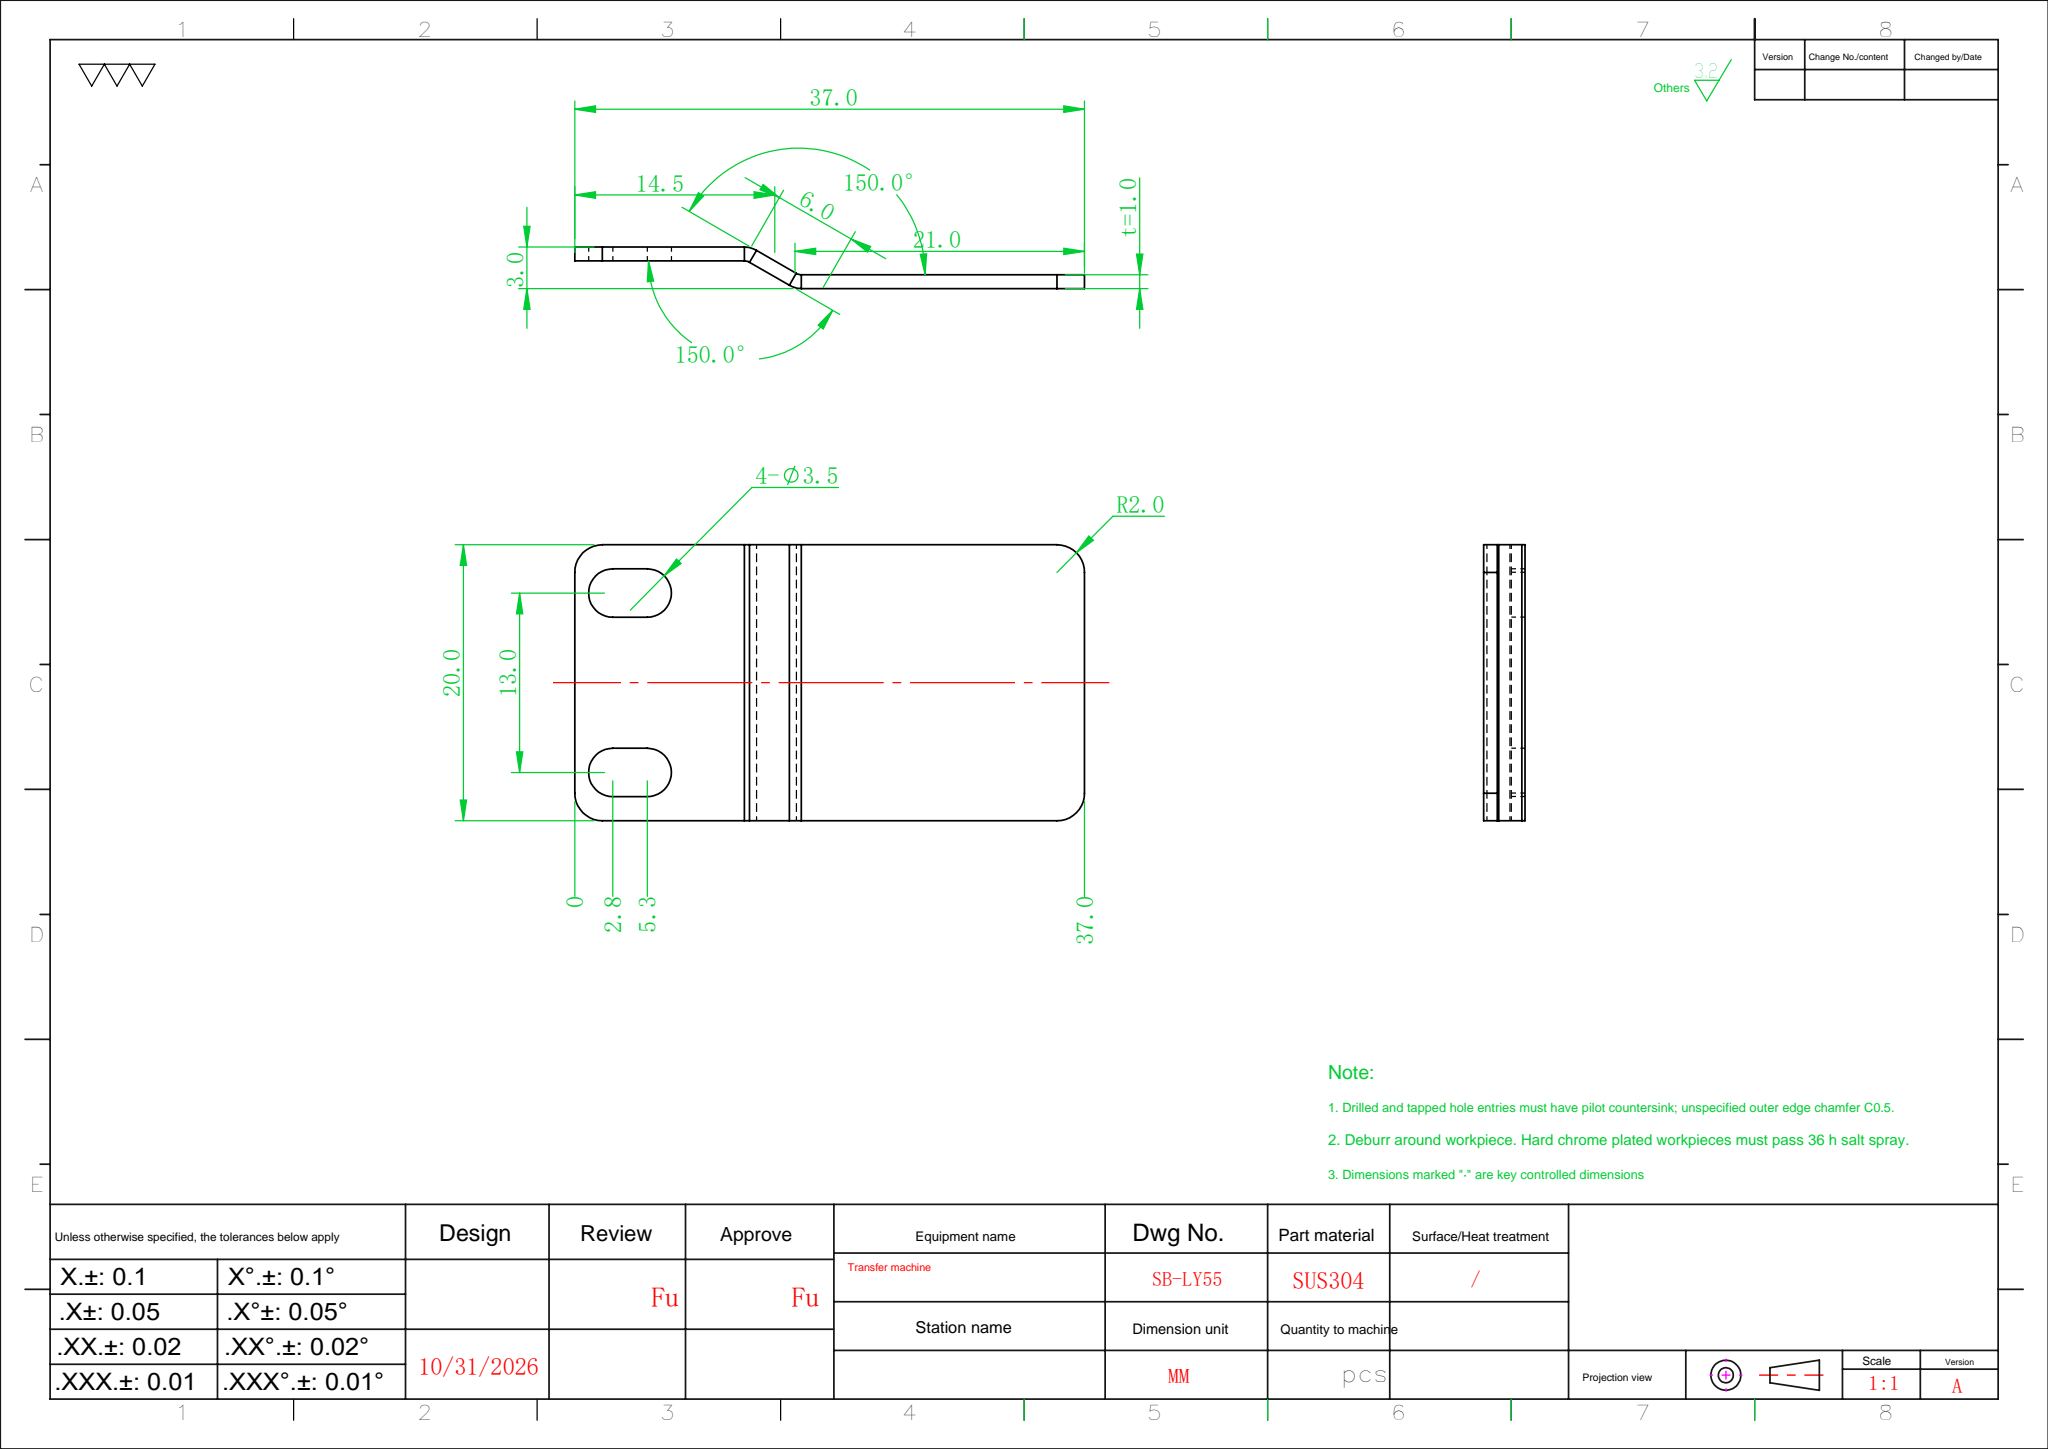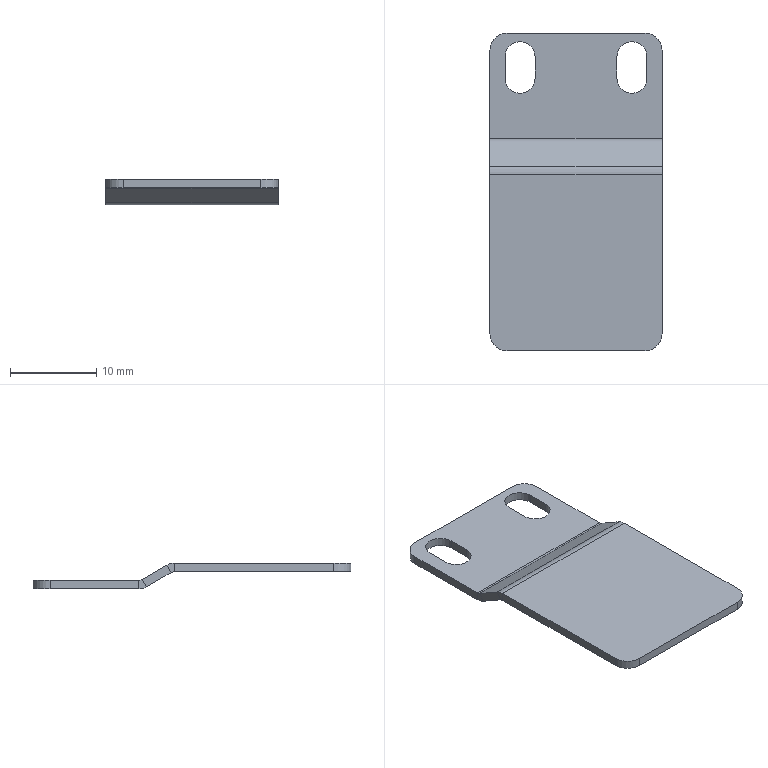Part | SolidWorks | features EdgeFlange 2, Fillet 1, FlatPattern 1, HoleWzd 1, SMBaseFlange 1, SheetMetal 1 | 1 solid | 34 faces | box 20 x 36.964 x 3 mm | volume 709.216 mm3 | plane 22 | cylinder 12 | commonest cylinder face diameters 3.5 x4 4 x4 1.473 x2 3.473 x2
STEP:
#1=CARTESIAN_POINT('',(-10.,-8.811,0.9013));
#2=VERTEX_POINT('',#1);
#3=CARTESIAN_POINT('',(-10.,-8.311,1.767));
#4=VERTEX_POINT('',#3);
#5=CARTESIAN_POINT('',(-10.,-8.811,0.9013));
#6=DIRECTION('',(0.,0.5,0.866));
#7=VECTOR('',#6,1000.);
#8=LINE('',#5,#7);
#9=EDGE_CURVE('',#2,#4,#8,.T.);
#10=ORIENTED_EDGE('',*,*,#9,.T.);
#11=CARTESIAN_POINT('',(-10.,-5.421,0.09869));
#12=VERTEX_POINT('',#11);
#13=CARTESIAN_POINT('',(-10.,-5.25,0.));
#14=DIRECTION('',(0.,0.866,-0.5));
#15=VECTOR('',#14,1000.);
#16=LINE('',#13,#15);
#17=EDGE_CURVE('',#4,#12,#16,.T.);
#18=ORIENTED_EDGE('',*,*,#17,.T.);
#19=CARTESIAN_POINT('',(-10.,-5.921,-0.7673));
#20=VERTEX_POINT('',#19);
#21=CARTESIAN_POINT('',(-10.,-5.921,-0.7673));
#22=DIRECTION('',(0.,-0.5,-0.866));
#23=VECTOR('',#22,1000.);
#24=LINE('',#21,#23);
#25=EDGE_CURVE('',#12,#20,#24,.T.);
#26=ORIENTED_EDGE('',*,*,#25,.T.);
#27=CARTESIAN_POINT('',(-10.,-0.3125,-4.005));
#28=DIRECTION('',(0.,0.866,-0.5));
#29=VECTOR('',#28,1000.);
#30=LINE('',#27,#29);
#31=EDGE_CURVE('',#2,#20,#30,.T.);
#32=ORIENTED_EDGE('',*,*,#31,.F.);
#33=EDGE_LOOP('',(#10,#18,#26,#32));
#34=FACE_OUTER_BOUND('',#33,.T.);
#35=CARTESIAN_POINT('',(-10.,-5.75,-0.866));
#36=DIRECTION('',(1.,0.,0.));
#37=DIRECTION('',(0.,0.,-1.));
#38=AXIS2_PLACEMENT_3D('',#35,#36,#37);
#39=PLANE('',#38);
#40=ADVANCED_FACE('',(#34),#39,.F.);
#41=CARTESIAN_POINT('',(10.,-8.811,0.9013));
#42=VERTEX_POINT('',#41);
#43=CARTESIAN_POINT('',(10.,-8.311,1.767));
#44=VERTEX_POINT('',#43);
#45=CARTESIAN_POINT('',(10.,-8.811,0.9013));
#46=DIRECTION('',(0.,0.5,0.866));
#47=VECTOR('',#46,1000.);
#48=LINE('',#45,#47);
#49=EDGE_CURVE('',#42,#44,#48,.T.);
#50=ORIENTED_EDGE('',*,*,#49,.F.);
#51=CARTESIAN_POINT('',(10.,-5.921,-0.7673));
#52=VERTEX_POINT('',#51);
#53=CARTESIAN_POINT('',(10.,-0.3125,-4.005));
#54=DIRECTION('',(0.,-0.866,0.5));
#55=VECTOR('',#54,1000.);
#56=LINE('',#53,#55);
#57=EDGE_CURVE('',#52,#42,#56,.T.);
#58=ORIENTED_EDGE('',*,*,#57,.F.);
#59=CARTESIAN_POINT('',(10.,-5.421,0.09869));
#60=VERTEX_POINT('',#59);
#61=CARTESIAN_POINT('',(10.,-5.421,0.09869));
#62=DIRECTION('',(0.,-0.5,-0.866));
#63=VECTOR('',#62,1000.);
#64=LINE('',#61,#63);
#65=EDGE_CURVE('',#60,#52,#64,.T.);
#66=ORIENTED_EDGE('',*,*,#65,.F.);
#67=CARTESIAN_POINT('',(10.,-10.214,2.866));
#68=DIRECTION('',(0.,-0.866,0.5));
#69=VECTOR('',#68,1000.);
#70=LINE('',#67,#69);
#71=EDGE_CURVE('',#60,#44,#70,.T.);
#72=ORIENTED_EDGE('',*,*,#71,.T.);
#73=EDGE_LOOP('',(#50,#58,#66,#72));
#74=FACE_OUTER_BOUND('',#73,.T.);
#75=CARTESIAN_POINT('',(10.,-10.714,2.));
#76=DIRECTION('',(-1.,0.,0.));
#77=DIRECTION('',(0.,0.,1.));
#78=AXIS2_PLACEMENT_3D('',#75,#76,#77);
#79=PLANE('',#78);
#80=ADVANCED_FACE('',(#74),#79,.F.);
#81=CARTESIAN_POINT('',(-10.,-8.811,0.9013));
#82=DIRECTION('',(1.,0.,0.));
#83=VECTOR('',#82,1000.);
#84=LINE('',#81,#83);
#85=EDGE_CURVE('',#2,#42,#84,.T.);
#86=ORIENTED_EDGE('',*,*,#85,.F.);
#87=ORIENTED_EDGE('',*,*,#31,.T.);
#88=CARTESIAN_POINT('',(-10.,-5.921,-0.7673));
#89=DIRECTION('',(-1.,0.,0.));
#90=VECTOR('',#89,1000.);
#91=LINE('',#88,#90);
#92=EDGE_CURVE('',#52,#20,#91,.T.);
#93=ORIENTED_EDGE('',*,*,#92,.F.);
#94=ORIENTED_EDGE('',*,*,#57,.T.);
#95=EDGE_LOOP('',(#86,#87,#93,#94));
#96=FACE_OUTER_BOUND('',#95,.T.);
#97=CARTESIAN_POINT('',(0.,-0.3125,-4.005));
#98=DIRECTION('',(0.,0.5,0.866));
#99=DIRECTION('',(0.,-0.866,0.5));
#100=AXIS2_PLACEMENT_3D('',#97,#98,#99);
#101=PLANE('',#100);
#102=ADVANCED_FACE('',(#96),#101,.F.);
#103=ORIENTED_EDGE('',*,*,#17,.F.);
#104=CARTESIAN_POINT('',(-10.,-8.311,1.767));
#105=DIRECTION('',(1.,0.,0.));
#106=VECTOR('',#105,1000.);
#107=LINE('',#104,#106);
#108=EDGE_CURVE('',#4,#44,#107,.T.);
#109=ORIENTED_EDGE('',*,*,#108,.T.);
#110=ORIENTED_EDGE('',*,*,#71,.F.);
#111=CARTESIAN_POINT('',(-10.,-5.421,0.09869));
#112=DIRECTION('',(1.,0.,0.));
#113=VECTOR('',#112,1000.);
#114=LINE('',#111,#113);
#115=EDGE_CURVE('',#12,#60,#114,.T.);
#116=ORIENTED_EDGE('',*,*,#115,.F.);
#117=EDGE_LOOP('',(#103,#109,#110,#116));
#118=FACE_OUTER_BOUND('',#117,.T.);
#119=CARTESIAN_POINT('',(0.,0.1875,-3.139));
#120=DIRECTION('',(0.,0.5,0.866));
#121=DIRECTION('',(0.,-0.866,0.5));
#122=AXIS2_PLACEMENT_3D('',#119,#120,#121);
#123=PLANE('',#122);
#124=ADVANCED_FACE('',(#118),#123,.T.);
#125=CARTESIAN_POINT('',(-4.75,4.5,0.));
#126=VERTEX_POINT('',#125);
#127=CARTESIAN_POINT('',(-8.25,4.5,0.));
#128=VERTEX_POINT('',#127);
#129=CARTESIAN_POINT('',(-6.5,4.5,0.));
#130=DIRECTION('',(0.,0.,1.));
#131=DIRECTION('',(1.,0.,0.));
#132=AXIS2_PLACEMENT_3D('',#129,#130,#131);
#133=CIRCLE('',#132,1.75);
#134=EDGE_CURVE('',#126,#128,#133,.T.);
#135=ORIENTED_EDGE('',*,*,#134,.F.);
#136=CARTESIAN_POINT('',(-4.75,2.,0.));
#137=VERTEX_POINT('',#136);
#138=CARTESIAN_POINT('',(-4.75,2.,0.));
#139=DIRECTION('',(0.,1.,0.));
#140=VECTOR('',#139,1000.);
#141=LINE('',#138,#140);
#142=EDGE_CURVE('',#137,#126,#141,.T.);
#143=ORIENTED_EDGE('',*,*,#142,.F.);
#144=CARTESIAN_POINT('',(-8.25,2.,0.));
#145=VERTEX_POINT('',#144);
#146=CARTESIAN_POINT('',(-6.5,2.,0.));
#147=DIRECTION('',(0.,0.,1.));
#148=DIRECTION('',(1.,0.,0.));
#149=AXIS2_PLACEMENT_3D('',#146,#147,#148);
#150=CIRCLE('',#149,1.75);
#151=EDGE_CURVE('',#145,#137,#150,.T.);
#152=ORIENTED_EDGE('',*,*,#151,.F.);
#153=CARTESIAN_POINT('',(-8.25,2.,0.));
#154=DIRECTION('',(0.,1.,0.));
#155=VECTOR('',#154,1000.);
#156=LINE('',#153,#155);
#157=EDGE_CURVE('',#145,#128,#156,.T.);
#158=ORIENTED_EDGE('',*,*,#157,.T.);
#159=EDGE_LOOP('',(#135,#143,#152,#158));
#160=FACE_BOUND('',#159,.T.);
#161=CARTESIAN_POINT('',(8.25,4.5,0.));
#162=VERTEX_POINT('',#161);
#163=CARTESIAN_POINT('',(4.75,4.5,0.));
#164=VERTEX_POINT('',#163);
#165=CARTESIAN_POINT('',(6.5,4.5,0.));
#166=DIRECTION('',(0.,0.,1.));
#167=DIRECTION('',(1.,0.,0.));
#168=AXIS2_PLACEMENT_3D('',#165,#166,#167);
#169=CIRCLE('',#168,1.75);
#170=EDGE_CURVE('',#162,#164,#169,.T.);
#171=ORIENTED_EDGE('',*,*,#170,.F.);
#172=CARTESIAN_POINT('',(8.25,2.,0.));
#173=VERTEX_POINT('',#172);
#174=CARTESIAN_POINT('',(8.25,2.,0.));
#175=DIRECTION('',(0.,1.,0.));
#176=VECTOR('',#175,1000.);
#177=LINE('',#174,#176);
#178=EDGE_CURVE('',#173,#162,#177,.T.);
#179=ORIENTED_EDGE('',*,*,#178,.F.);
#180=CARTESIAN_POINT('',(4.75,2.,0.));
#181=VERTEX_POINT('',#180);
#182=CARTESIAN_POINT('',(6.5,2.,0.));
#183=DIRECTION('',(0.,0.,1.));
#184=DIRECTION('',(1.,0.,0.));
#185=AXIS2_PLACEMENT_3D('',#182,#183,#184);
#186=CIRCLE('',#185,1.75);
#187=EDGE_CURVE('',#181,#173,#186,.T.);
#188=ORIENTED_EDGE('',*,*,#187,.F.);
#189=CARTESIAN_POINT('',(4.75,2.,0.));
#190=DIRECTION('',(0.,1.,0.));
#191=VECTOR('',#190,1000.);
#192=LINE('',#189,#191);
#193=EDGE_CURVE('',#181,#164,#192,.T.);
#194=ORIENTED_EDGE('',*,*,#193,.T.);
#195=EDGE_LOOP('',(#171,#179,#188,#194));
#196=FACE_BOUND('',#195,.T.);
#197=CARTESIAN_POINT('',(8.,7.25,0.));
#198=VERTEX_POINT('',#197);
#199=CARTESIAN_POINT('',(-8.,7.25,0.));
#200=VERTEX_POINT('',#199);
#201=CARTESIAN_POINT('',(-10.,7.25,0.));
#202=DIRECTION('',(-1.,0.,0.));
#203=VECTOR('',#202,1000.);
#204=LINE('',#201,#203);
#205=EDGE_CURVE('',#198,#200,#204,.T.);
#206=ORIENTED_EDGE('',*,*,#205,.T.);
#207=CARTESIAN_POINT('',(-10.,5.25,0.));
#208=VERTEX_POINT('',#207);
#209=CARTESIAN_POINT('',(-8.,5.25,0.));
#210=DIRECTION('',(0.,0.,1.));
#211=DIRECTION('',(-1.,0.,0.));
#212=AXIS2_PLACEMENT_3D('',#209,#210,#211);
#213=CIRCLE('',#212,2.);
#214=EDGE_CURVE('',#200,#208,#213,.T.);
#215=ORIENTED_EDGE('',*,*,#214,.T.);
#216=CARTESIAN_POINT('',(-10.,-5.053,0.));
#217=VERTEX_POINT('',#216);
#218=CARTESIAN_POINT('',(-10.,-7.25,0.));
#219=DIRECTION('',(0.,-1.,0.));
#220=VECTOR('',#219,1000.);
#221=LINE('',#218,#220);
#222=EDGE_CURVE('',#208,#217,#221,.T.);
#223=ORIENTED_EDGE('',*,*,#222,.T.);
#224=CARTESIAN_POINT('',(10.,-5.053,0.));
#225=VERTEX_POINT('',#224);
#226=CARTESIAN_POINT('',(10.,-5.053,0.));
#227=DIRECTION('',(-1.,0.,0.));
#228=VECTOR('',#227,1000.);
#229=LINE('',#226,#228);
#230=EDGE_CURVE('',#225,#217,#229,.T.);
#231=ORIENTED_EDGE('',*,*,#230,.F.);
#232=CARTESIAN_POINT('',(10.,5.25,0.));
#233=VERTEX_POINT('',#232);
#234=CARTESIAN_POINT('',(10.,-7.25,0.));
#235=DIRECTION('',(0.,1.,0.));
#236=VECTOR('',#235,1000.);
#237=LINE('',#234,#236);
#238=EDGE_CURVE('',#225,#233,#237,.T.);
#239=ORIENTED_EDGE('',*,*,#238,.T.);
#240=CARTESIAN_POINT('',(8.,5.25,0.));
#241=DIRECTION('',(0.,0.,1.));
#242=DIRECTION('',(-1.,0.,0.));
#243=AXIS2_PLACEMENT_3D('',#240,#241,#242);
#244=CIRCLE('',#243,2.);
#245=EDGE_CURVE('',#233,#198,#244,.T.);
#246=ORIENTED_EDGE('',*,*,#245,.T.);
#247=EDGE_LOOP('',(#206,#215,#223,#231,#239,#246));
#248=FACE_OUTER_BOUND('',#247,.T.);
#249=CARTESIAN_POINT('',(0.,0.,0.));
#250=DIRECTION('',(0.,0.,-1.));
#251=DIRECTION('',(-1.,0.,0.));
#252=AXIS2_PLACEMENT_3D('',#249,#250,#251);
#253=PLANE('',#252);
#254=ADVANCED_FACE('',(#160,#196,#248),#253,.F.);
#255=CARTESIAN_POINT('',(10.,-5.053,-1.));
#256=VERTEX_POINT('',#255);
#257=CARTESIAN_POINT('',(10.,5.25,-1.));
#258=VERTEX_POINT('',#257);
#259=CARTESIAN_POINT('',(10.,-7.25,-1.));
#260=DIRECTION('',(0.,1.,0.));
#261=VECTOR('',#260,1000.);
#262=LINE('',#259,#261);
#263=EDGE_CURVE('',#256,#258,#262,.T.);
#264=ORIENTED_EDGE('',*,*,#263,.T.);
#265=CARTESIAN_POINT('',(10.,5.25,-1.));
#266=DIRECTION('',(0.,0.,1.));
#267=VECTOR('',#266,1000.);
#268=LINE('',#265,#267);
#269=EDGE_CURVE('',#258,#233,#268,.T.);
#270=ORIENTED_EDGE('',*,*,#269,.T.);
#271=ORIENTED_EDGE('',*,*,#238,.F.);
#272=CARTESIAN_POINT('',(10.,-5.053,0.));
#273=DIRECTION('',(0.,0.,-1.));
#274=VECTOR('',#273,1000.);
#275=LINE('',#272,#274);
#276=EDGE_CURVE('',#225,#256,#275,.T.);
#277=ORIENTED_EDGE('',*,*,#276,.T.);
#278=EDGE_LOOP('',(#264,#270,#271,#277));
#279=FACE_OUTER_BOUND('',#278,.T.);
#280=CARTESIAN_POINT('',(10.,-7.25,-1.));
#281=DIRECTION('',(1.,0.,0.));
#282=DIRECTION('',(0.,0.,-1.));
#283=AXIS2_PLACEMENT_3D('',#280,#281,#282);
#284=PLANE('',#283);
#285=ADVANCED_FACE('',(#279),#284,.T.);
#286=CARTESIAN_POINT('',(-4.75,2.,-1.));
#287=VERTEX_POINT('',#286);
#288=CARTESIAN_POINT('',(-4.75,4.5,-1.));
#289=VERTEX_POINT('',#288);
#290=CARTESIAN_POINT('',(-4.75,2.,-1.));
#291=DIRECTION('',(0.,1.,0.));
#292=VECTOR('',#291,1000.);
#293=LINE('',#290,#292);
#294=EDGE_CURVE('',#287,#289,#293,.T.);
#295=ORIENTED_EDGE('',*,*,#294,.T.);
#296=CARTESIAN_POINT('',(-8.25,4.5,-1.));
#297=VERTEX_POINT('',#296);
#298=CARTESIAN_POINT('',(-6.5,4.5,-1.));
#299=DIRECTION('',(0.,0.,1.));
#300=DIRECTION('',(1.,0.,0.));
#301=AXIS2_PLACEMENT_3D('',#298,#299,#300);
#302=CIRCLE('',#301,1.75);
#303=EDGE_CURVE('',#289,#297,#302,.T.);
#304=ORIENTED_EDGE('',*,*,#303,.T.);
#305=CARTESIAN_POINT('',(-8.25,2.,-1.));
#306=VERTEX_POINT('',#305);
#307=CARTESIAN_POINT('',(-8.25,2.,-1.));
#308=DIRECTION('',(0.,1.,0.));
#309=VECTOR('',#308,1000.);
#310=LINE('',#307,#309);
#311=EDGE_CURVE('',#306,#297,#310,.T.);
#312=ORIENTED_EDGE('',*,*,#311,.F.);
#313=CARTESIAN_POINT('',(-6.5,2.,-1.));
#314=DIRECTION('',(0.,0.,1.));
#315=DIRECTION('',(1.,0.,0.));
#316=AXIS2_PLACEMENT_3D('',#313,#314,#315);
#317=CIRCLE('',#316,1.75);
#318=EDGE_CURVE('',#306,#287,#317,.T.);
#319=ORIENTED_EDGE('',*,*,#318,.T.);
#320=EDGE_LOOP('',(#295,#304,#312,#319));
#321=FACE_BOUND('',#320,.T.);
#322=CARTESIAN_POINT('',(4.75,2.,-1.));
#323=VERTEX_POINT('',#322);
#324=CARTESIAN_POINT('',(4.75,4.5,-1.));
#325=VERTEX_POINT('',#324);
#326=CARTESIAN_POINT('',(4.75,2.,-1.));
#327=DIRECTION('',(0.,1.,0.));
#328=VECTOR('',#327,1000.);
#329=LINE('',#326,#328);
#330=EDGE_CURVE('',#323,#325,#329,.T.);
#331=ORIENTED_EDGE('',*,*,#330,.F.);
#332=CARTESIAN_POINT('',(8.25,2.,-1.));
#333=VERTEX_POINT('',#332);
#334=CARTESIAN_POINT('',(6.5,2.,-1.));
#335=DIRECTION('',(0.,0.,1.));
#336=DIRECTION('',(1.,0.,0.));
#337=AXIS2_PLACEMENT_3D('',#334,#335,#336);
#338=CIRCLE('',#337,1.75);
#339=EDGE_CURVE('',#323,#333,#338,.T.);
#340=ORIENTED_EDGE('',*,*,#339,.T.);
#341=CARTESIAN_POINT('',(8.25,4.5,-1.));
#342=VERTEX_POINT('',#341);
#343=CARTESIAN_POINT('',(8.25,2.,-1.));
#344=DIRECTION('',(0.,1.,0.));
#345=VECTOR('',#344,1000.);
#346=LINE('',#343,#345);
#347=EDGE_CURVE('',#333,#342,#346,.T.);
#348=ORIENTED_EDGE('',*,*,#347,.T.);
#349=CARTESIAN_POINT('',(6.5,4.5,-1.));
#350=DIRECTION('',(0.,0.,1.));
#351=DIRECTION('',(1.,0.,0.));
#352=AXIS2_PLACEMENT_3D('',#349,#350,#351);
#353=CIRCLE('',#352,1.75);
#354=EDGE_CURVE('',#342,#325,#353,.T.);
#355=ORIENTED_EDGE('',*,*,#354,.T.);
#356=EDGE_LOOP('',(#331,#340,#348,#355));
#357=FACE_BOUND('',#356,.T.);
#358=CARTESIAN_POINT('',(-10.,5.25,-1.));
#359=VERTEX_POINT('',#358);
#360=CARTESIAN_POINT('',(-10.,-5.053,-1.));
#361=VERTEX_POINT('',#360);
#362=CARTESIAN_POINT('',(-10.,-7.25,-1.));
#363=DIRECTION('',(0.,-1.,0.));
#364=VECTOR('',#363,1000.);
#365=LINE('',#362,#364);
#366=EDGE_CURVE('',#359,#361,#365,.T.);
#367=ORIENTED_EDGE('',*,*,#366,.F.);
#368=CARTESIAN_POINT('',(-8.,7.25,-1.));
#369=VERTEX_POINT('',#368);
#370=CARTESIAN_POINT('',(-8.,5.25,-1.));
#371=DIRECTION('',(0.,0.,-1.));
#372=DIRECTION('',(-1.,0.,0.));
#373=AXIS2_PLACEMENT_3D('',#370,#371,#372);
#374=CIRCLE('',#373,2.);
#375=EDGE_CURVE('',#359,#369,#374,.T.);
#376=ORIENTED_EDGE('',*,*,#375,.T.);
#377=CARTESIAN_POINT('',(8.,7.25,-1.));
#378=VERTEX_POINT('',#377);
#379=CARTESIAN_POINT('',(-10.,7.25,-1.));
#380=DIRECTION('',(-1.,0.,0.));
#381=VECTOR('',#380,1000.);
#382=LINE('',#379,#381);
#383=EDGE_CURVE('',#378,#369,#382,.T.);
#384=ORIENTED_EDGE('',*,*,#383,.F.);
#385=CARTESIAN_POINT('',(8.,5.25,-1.));
#386=DIRECTION('',(0.,0.,-1.));
#387=DIRECTION('',(-1.,0.,0.));
#388=AXIS2_PLACEMENT_3D('',#385,#386,#387);
#389=CIRCLE('',#388,2.);
#390=EDGE_CURVE('',#378,#258,#389,.T.);
#391=ORIENTED_EDGE('',*,*,#390,.T.);
#392=ORIENTED_EDGE('',*,*,#263,.F.);
#393=CARTESIAN_POINT('',(10.,-5.053,-1.));
#394=DIRECTION('',(-1.,0.,0.));
#395=VECTOR('',#394,1000.);
#396=LINE('',#393,#395);
#397=EDGE_CURVE('',#256,#361,#396,.T.);
#398=ORIENTED_EDGE('',*,*,#397,.T.);
#399=EDGE_LOOP('',(#367,#376,#384,#391,#392,#398));
#400=FACE_OUTER_BOUND('',#399,.T.);
#401=CARTESIAN_POINT('',(0.,0.,-1.));
#402=DIRECTION('',(0.,0.,-1.));
#403=DIRECTION('',(-1.,0.,0.));
#404=AXIS2_PLACEMENT_3D('',#401,#402,#403);
#405=PLANE('',#404);
#406=ADVANCED_FACE('',(#321,#357,#400),#405,.T.);
#407=ORIENTED_EDGE('',*,*,#222,.F.);
#408=CARTESIAN_POINT('',(-10.,5.25,-1.));
#409=DIRECTION('',(0.,0.,-1.));
#410=VECTOR('',#409,1000.);
#411=LINE('',#408,#410);
#412=EDGE_CURVE('',#208,#359,#411,.T.);
#413=ORIENTED_EDGE('',*,*,#412,.T.);
#414=ORIENTED_EDGE('',*,*,#366,.T.);
#415=CARTESIAN_POINT('',(-10.,-5.053,0.));
#416=DIRECTION('',(0.,0.,-1.));
#417=VECTOR('',#416,1000.);
#418=LINE('',#415,#417);
#419=EDGE_CURVE('',#217,#361,#418,.T.);
#420=ORIENTED_EDGE('',*,*,#419,.F.);
#421=EDGE_LOOP('',(#407,#413,#414,#420));
#422=FACE_OUTER_BOUND('',#421,.T.);
#423=CARTESIAN_POINT('',(-10.,-7.25,-1.));
#424=DIRECTION('',(-1.,0.,0.));
#425=DIRECTION('',(0.,0.,1.));
#426=AXIS2_PLACEMENT_3D('',#423,#424,#425);
#427=PLANE('',#426);
#428=ADVANCED_FACE('',(#422),#427,.T.);
#429=ORIENTED_EDGE('',*,*,#383,.T.);
#430=CARTESIAN_POINT('',(-8.,7.25,-1.));
#431=DIRECTION('',(0.,0.,1.));
#432=VECTOR('',#431,1000.);
#433=LINE('',#430,#432);
#434=EDGE_CURVE('',#369,#200,#433,.T.);
#435=ORIENTED_EDGE('',*,*,#434,.T.);
#436=ORIENTED_EDGE('',*,*,#205,.F.);
#437=CARTESIAN_POINT('',(8.,7.25,-1.));
#438=DIRECTION('',(0.,0.,-1.));
#439=VECTOR('',#438,1000.);
#440=LINE('',#437,#439);
#441=EDGE_CURVE('',#198,#378,#440,.T.);
#442=ORIENTED_EDGE('',*,*,#441,.T.);
#443=EDGE_LOOP('',(#429,#435,#436,#442));
#444=FACE_OUTER_BOUND('',#443,.T.);
#445=CARTESIAN_POINT('',(-10.,7.25,-1.));
#446=DIRECTION('',(0.,1.,0.));
#447=DIRECTION('',(0.,0.,1.));
#448=AXIS2_PLACEMENT_3D('',#445,#446,#447);
#449=PLANE('',#448);
#450=ADVANCED_FACE('',(#444),#449,.T.);
#451=ORIENTED_EDGE('',*,*,#354,.F.);
#452=CARTESIAN_POINT('',(8.25,4.5,-1.));
#453=DIRECTION('',(0.,0.,-1.));
#454=VECTOR('',#453,1000.);
#455=LINE('',#452,#454);
#456=EDGE_CURVE('',#162,#342,#455,.T.);
#457=ORIENTED_EDGE('',*,*,#456,.F.);
#458=ORIENTED_EDGE('',*,*,#170,.T.);
#459=CARTESIAN_POINT('',(4.75,4.5,0.));
#460=DIRECTION('',(0.,0.,1.));
#461=VECTOR('',#460,1000.);
#462=LINE('',#459,#461);
#463=EDGE_CURVE('',#325,#164,#462,.T.);
#464=ORIENTED_EDGE('',*,*,#463,.F.);
#465=EDGE_LOOP('',(#451,#457,#458,#464));
#466=FACE_OUTER_BOUND('',#465,.T.);
#467=CARTESIAN_POINT('',(6.5,4.5,0.));
#468=DIRECTION('',(0.,0.,1.));
#469=DIRECTION('',(1.,0.,0.));
#470=AXIS2_PLACEMENT_3D('',#467,#468,#469);
#471=CYLINDRICAL_SURFACE('',#470,1.75);
#472=ADVANCED_FACE('',(#466),#471,.F.);
#473=ORIENTED_EDGE('',*,*,#187,.T.);
#474=CARTESIAN_POINT('',(8.25,2.,-1.));
#475=DIRECTION('',(0.,0.,-1.));
#476=VECTOR('',#475,1000.);
#477=LINE('',#474,#476);
#478=EDGE_CURVE('',#173,#333,#477,.T.);
#479=ORIENTED_EDGE('',*,*,#478,.T.);
#480=ORIENTED_EDGE('',*,*,#339,.F.);
#481=CARTESIAN_POINT('',(4.75,2.,0.));
#482=DIRECTION('',(0.,0.,-1.));
#483=VECTOR('',#482,1000.);
#484=LINE('',#481,#483);
#485=EDGE_CURVE('',#181,#323,#484,.T.);
#486=ORIENTED_EDGE('',*,*,#485,.F.);
#487=EDGE_LOOP('',(#473,#479,#480,#486));
#488=FACE_OUTER_BOUND('',#487,.T.);
#489=CARTESIAN_POINT('',(6.5,2.,0.));
#490=DIRECTION('',(0.,0.,1.));
#491=DIRECTION('',(1.,0.,0.));
#492=AXIS2_PLACEMENT_3D('',#489,#490,#491);
#493=CYLINDRICAL_SURFACE('',#492,1.75);
#494=ADVANCED_FACE('',(#488),#493,.F.);
#495=ORIENTED_EDGE('',*,*,#463,.T.);
#496=ORIENTED_EDGE('',*,*,#193,.F.);
#497=ORIENTED_EDGE('',*,*,#485,.T.);
#498=ORIENTED_EDGE('',*,*,#330,.T.);
#499=EDGE_LOOP('',(#495,#496,#497,#498));
#500=FACE_OUTER_BOUND('',#499,.T.);
#501=CARTESIAN_POINT('',(4.75,2.,0.));
#502=DIRECTION('',(-1.,0.,0.));
#503=DIRECTION('',(0.,0.,1.));
#504=AXIS2_PLACEMENT_3D('',#501,#502,#503);
#505=PLANE('',#504);
#506=ADVANCED_FACE('',(#500),#505,.F.);
#507=ORIENTED_EDGE('',*,*,#456,.T.);
#508=ORIENTED_EDGE('',*,*,#347,.F.);
#509=ORIENTED_EDGE('',*,*,#478,.F.);
#510=ORIENTED_EDGE('',*,*,#178,.T.);
#511=EDGE_LOOP('',(#507,#508,#509,#510));
#512=FACE_OUTER_BOUND('',#511,.T.);
#513=CARTESIAN_POINT('',(8.25,2.,-1.));
#514=DIRECTION('',(1.,0.,0.));
#515=DIRECTION('',(0.,0.,-1.));
#516=AXIS2_PLACEMENT_3D('',#513,#514,#515);
#517=PLANE('',#516);
#518=ADVANCED_FACE('',(#512),#517,.F.);
#519=ORIENTED_EDGE('',*,*,#303,.F.);
#520=CARTESIAN_POINT('',(-4.75,4.5,-1.));
#521=DIRECTION('',(0.,0.,-1.));
#522=VECTOR('',#521,1000.);
#523=LINE('',#520,#522);
#524=EDGE_CURVE('',#126,#289,#523,.T.);
#525=ORIENTED_EDGE('',*,*,#524,.F.);
#526=ORIENTED_EDGE('',*,*,#134,.T.);
#527=CARTESIAN_POINT('',(-8.25,4.5,0.));
#528=DIRECTION('',(0.,0.,1.));
#529=VECTOR('',#528,1000.);
#530=LINE('',#527,#529);
#531=EDGE_CURVE('',#297,#128,#530,.T.);
#532=ORIENTED_EDGE('',*,*,#531,.F.);
#533=EDGE_LOOP('',(#519,#525,#526,#532));
#534=FACE_OUTER_BOUND('',#533,.T.);
#535=CARTESIAN_POINT('',(-6.5,4.5,0.));
#536=DIRECTION('',(0.,0.,1.));
#537=DIRECTION('',(1.,0.,0.));
#538=AXIS2_PLACEMENT_3D('',#535,#536,#537);
#539=CYLINDRICAL_SURFACE('',#538,1.75);
#540=ADVANCED_FACE('',(#534),#539,.F.);
#541=ORIENTED_EDGE('',*,*,#151,.T.);
#542=CARTESIAN_POINT('',(-4.75,2.,-1.));
#543=DIRECTION('',(0.,0.,-1.));
#544=VECTOR('',#543,1000.);
#545=LINE('',#542,#544);
#546=EDGE_CURVE('',#137,#287,#545,.T.);
#547=ORIENTED_EDGE('',*,*,#546,.T.);
#548=ORIENTED_EDGE('',*,*,#318,.F.);
#549=CARTESIAN_POINT('',(-8.25,2.,0.));
#550=DIRECTION('',(0.,0.,-1.));
#551=VECTOR('',#550,1000.);
#552=LINE('',#549,#551);
#553=EDGE_CURVE('',#145,#306,#552,.T.);
#554=ORIENTED_EDGE('',*,*,#553,.F.);
#555=EDGE_LOOP('',(#541,#547,#548,#554));
#556=FACE_OUTER_BOUND('',#555,.T.);
#557=CARTESIAN_POINT('',(-6.5,2.,0.));
#558=DIRECTION('',(0.,0.,1.));
#559=DIRECTION('',(1.,0.,0.));
#560=AXIS2_PLACEMENT_3D('',#557,#558,#559);
#561=CYLINDRICAL_SURFACE('',#560,1.75);
#562=ADVANCED_FACE('',(#556),#561,.F.);
#563=ORIENTED_EDGE('',*,*,#531,.T.);
#564=ORIENTED_EDGE('',*,*,#157,.F.);
#565=ORIENTED_EDGE('',*,*,#553,.T.);
#566=ORIENTED_EDGE('',*,*,#311,.T.);
#567=EDGE_LOOP('',(#563,#564,#565,#566));
#568=FACE_OUTER_BOUND('',#567,.T.);
#569=CARTESIAN_POINT('',(-8.25,2.,0.));
#570=DIRECTION('',(-1.,0.,0.));
#571=DIRECTION('',(0.,0.,1.));
#572=AXIS2_PLACEMENT_3D('',#569,#570,#571);
#573=PLANE('',#572);
#574=ADVANCED_FACE('',(#568),#573,.F.);
#575=ORIENTED_EDGE('',*,*,#524,.T.);
#576=ORIENTED_EDGE('',*,*,#294,.F.);
#577=ORIENTED_EDGE('',*,*,#546,.F.);
#578=ORIENTED_EDGE('',*,*,#142,.T.);
#579=EDGE_LOOP('',(#575,#576,#577,#578));
#580=FACE_OUTER_BOUND('',#579,.T.);
#581=CARTESIAN_POINT('',(-4.75,2.,-1.));
#582=DIRECTION('',(1.,0.,0.));
#583=DIRECTION('',(0.,0.,-1.));
#584=AXIS2_PLACEMENT_3D('',#581,#582,#583);
#585=PLANE('',#584);
#586=ADVANCED_FACE('',(#580),#585,.F.);
#587=ORIENTED_EDGE('',*,*,#25,.F.);
#588=CARTESIAN_POINT('',(-10.,-5.053,0.7366));
#589=DIRECTION('',(-1.,0.,0.));
#590=DIRECTION('',(0.,0.,-1.));
#591=AXIS2_PLACEMENT_3D('',#588,#589,#590);
#592=CIRCLE('',#591,0.7366);
#593=EDGE_CURVE('',#217,#12,#592,.T.);
#594=ORIENTED_EDGE('',*,*,#593,.F.);
#595=ORIENTED_EDGE('',*,*,#419,.T.);
#596=CARTESIAN_POINT('',(-10.,-5.053,0.7366));
#597=DIRECTION('',(-1.,0.,0.));
#598=DIRECTION('',(0.,0.,-1.));
#599=AXIS2_PLACEMENT_3D('',#596,#597,#598);
#600=CIRCLE('',#599,1.737);
#601=EDGE_CURVE('',#361,#20,#600,.T.);
#602=ORIENTED_EDGE('',*,*,#601,.T.);
#603=EDGE_LOOP('',(#587,#594,#595,#602));
#604=FACE_OUTER_BOUND('',#603,.T.);
#605=CARTESIAN_POINT('',(-10.,-5.053,0.7366));
#606=DIRECTION('',(-1.,0.,0.));
#607=DIRECTION('',(0.,0.,1.));
#608=AXIS2_PLACEMENT_3D('',#605,#606,#607);
#609=PLANE('',#608);
#610=ADVANCED_FACE('',(#604),#609,.T.);
#611=CARTESIAN_POINT('',(10.,-5.053,0.7366));
#612=DIRECTION('',(1.,0.,0.));
#613=DIRECTION('',(0.,0.,-1.));
#614=AXIS2_PLACEMENT_3D('',#611,#612,#613);
#615=CIRCLE('',#614,0.7366);
#616=EDGE_CURVE('',#60,#225,#615,.T.);
#617=ORIENTED_EDGE('',*,*,#616,.F.);
#618=ORIENTED_EDGE('',*,*,#65,.T.);
#619=CARTESIAN_POINT('',(10.,-5.053,0.7366));
#620=DIRECTION('',(1.,0.,0.));
#621=DIRECTION('',(0.,0.,-1.));
#622=AXIS2_PLACEMENT_3D('',#619,#620,#621);
#623=CIRCLE('',#622,1.737);
#624=EDGE_CURVE('',#52,#256,#623,.T.);
#625=ORIENTED_EDGE('',*,*,#624,.T.);
#626=ORIENTED_EDGE('',*,*,#276,.F.);
#627=EDGE_LOOP('',(#617,#618,#625,#626));
#628=FACE_OUTER_BOUND('',#627,.T.);
#629=CARTESIAN_POINT('',(10.,-5.053,0.7366));
#630=DIRECTION('',(-1.,0.,0.));
#631=DIRECTION('',(0.,0.,1.));
#632=AXIS2_PLACEMENT_3D('',#629,#630,#631);
#633=PLANE('',#632);
#634=ADVANCED_FACE('',(#628),#633,.F.);
#635=ORIENTED_EDGE('',*,*,#397,.F.);
#636=ORIENTED_EDGE('',*,*,#624,.F.);
#637=ORIENTED_EDGE('',*,*,#92,.T.);
#638=ORIENTED_EDGE('',*,*,#601,.F.);
#639=EDGE_LOOP('',(#635,#636,#637,#638));
#640=FACE_OUTER_BOUND('',#639,.T.);
#641=CARTESIAN_POINT('',(10.,-5.053,0.7366));
#642=DIRECTION('',(1.,0.,0.));
#643=DIRECTION('',(0.,-0.5,-0.866));
#644=AXIS2_PLACEMENT_3D('',#641,#642,#643);
#645=CYLINDRICAL_SURFACE('',#644,1.737);
#646=ADVANCED_FACE('',(#640),#645,.T.);
#647=ORIENTED_EDGE('',*,*,#230,.T.);
#648=ORIENTED_EDGE('',*,*,#593,.T.);
#649=ORIENTED_EDGE('',*,*,#115,.T.);
#650=ORIENTED_EDGE('',*,*,#616,.T.);
#651=EDGE_LOOP('',(#647,#648,#649,#650));
#652=FACE_OUTER_BOUND('',#651,.T.);
#653=CARTESIAN_POINT('',(10.,-5.053,0.7366));
#654=DIRECTION('',(1.,0.,0.));
#655=DIRECTION('',(0.,-0.5,-0.866));
#656=AXIS2_PLACEMENT_3D('',#653,#654,#655);
#657=CYLINDRICAL_SURFACE('',#656,0.7366);
#658=ADVANCED_FACE('',(#652),#657,.F.);
#659=CARTESIAN_POINT('',(10.,-9.179,1.));
#660=VERTEX_POINT('',#659);
#661=CARTESIAN_POINT('',(10.,-9.179,2.));
#662=VERTEX_POINT('',#661);
#663=CARTESIAN_POINT('',(10.,-9.179,2.));
#664=DIRECTION('',(0.,0.,1.));
#665=VECTOR('',#664,1000.);
#666=LINE('',#663,#665);
#667=EDGE_CURVE('',#660,#662,#666,.T.);
#668=ORIENTED_EDGE('',*,*,#667,.F.);
#669=CARTESIAN_POINT('',(10.,-9.179,0.2634));
#670=DIRECTION('',(1.,0.,0.));
#671=DIRECTION('',(0.,0.,1.));
#672=AXIS2_PLACEMENT_3D('',#669,#670,#671);
#673=CIRCLE('',#672,0.7366);
#674=EDGE_CURVE('',#42,#660,#673,.T.);
#675=ORIENTED_EDGE('',*,*,#674,.F.);
#676=ORIENTED_EDGE('',*,*,#49,.T.);
#677=CARTESIAN_POINT('',(10.,-9.179,0.2634));
#678=DIRECTION('',(1.,0.,0.));
#679=DIRECTION('',(0.,0.,1.));
#680=AXIS2_PLACEMENT_3D('',#677,#678,#679);
#681=CIRCLE('',#680,1.737);
#682=EDGE_CURVE('',#44,#662,#681,.T.);
#683=ORIENTED_EDGE('',*,*,#682,.T.);
#684=EDGE_LOOP('',(#668,#675,#676,#683));
#685=FACE_OUTER_BOUND('',#684,.T.);
#686=CARTESIAN_POINT('',(10.,-9.179,0.2634));
#687=DIRECTION('',(1.,0.,0.));
#688=DIRECTION('',(0.,0.,-1.));
#689=AXIS2_PLACEMENT_3D('',#686,#687,#688);
#690=PLANE('',#689);
#691=ADVANCED_FACE('',(#685),#690,.T.);
#692=CARTESIAN_POINT('',(-10.,-9.179,1.));
#693=VERTEX_POINT('',#692);
#694=CARTESIAN_POINT('',(-10.,-9.179,0.2634));
#695=DIRECTION('',(-1.,0.,0.));
#696=DIRECTION('',(0.,0.,1.));
#697=AXIS2_PLACEMENT_3D('',#694,#695,#696);
#698=CIRCLE('',#697,0.7366);
#699=EDGE_CURVE('',#693,#2,#698,.T.);
#700=ORIENTED_EDGE('',*,*,#699,.F.);
#701=CARTESIAN_POINT('',(-10.,-9.179,2.));
#702=VERTEX_POINT('',#701);
#703=CARTESIAN_POINT('',(-10.,-9.179,1.));
#704=DIRECTION('',(0.,0.,1.));
#705=VECTOR('',#704,1000.);
#706=LINE('',#703,#705);
#707=EDGE_CURVE('',#693,#702,#706,.T.);
#708=ORIENTED_EDGE('',*,*,#707,.T.);
#709=CARTESIAN_POINT('',(-10.,-9.179,0.2634));
#710=DIRECTION('',(-1.,0.,0.));
#711=DIRECTION('',(0.,0.,1.));
#712=AXIS2_PLACEMENT_3D('',#709,#710,#711);
#713=CIRCLE('',#712,1.737);
#714=EDGE_CURVE('',#702,#4,#713,.T.);
#715=ORIENTED_EDGE('',*,*,#714,.T.);
#716=ORIENTED_EDGE('',*,*,#9,.F.);
#717=EDGE_LOOP('',(#700,#708,#715,#716));
#718=FACE_OUTER_BOUND('',#717,.T.);
#719=CARTESIAN_POINT('',(-10.,-9.179,0.2634));
#720=DIRECTION('',(1.,0.,0.));
#721=DIRECTION('',(0.,0.,-1.));
#722=AXIS2_PLACEMENT_3D('',#719,#720,#721);
#723=PLANE('',#722);
#724=ADVANCED_FACE('',(#718),#723,.F.);
#725=ORIENTED_EDGE('',*,*,#108,.F.);
#726=ORIENTED_EDGE('',*,*,#714,.F.);
#727=CARTESIAN_POINT('',(0.,-9.179,2.));
#728=DIRECTION('',(-1.,0.,0.));
#729=VECTOR('',#728,1000.);
#730=LINE('',#727,#729);
#731=EDGE_CURVE('',#662,#702,#730,.T.);
#732=ORIENTED_EDGE('',*,*,#731,.F.);
#733=ORIENTED_EDGE('',*,*,#682,.F.);
#734=EDGE_LOOP('',(#725,#726,#732,#733));
#735=FACE_OUTER_BOUND('',#734,.T.);
#736=CARTESIAN_POINT('',(-10.,-9.179,0.2634));
#737=DIRECTION('',(-1.,0.,0.));
#738=DIRECTION('',(0.,0.,1.));
#739=AXIS2_PLACEMENT_3D('',#736,#737,#738);
#740=CYLINDRICAL_SURFACE('',#739,1.737);
#741=ADVANCED_FACE('',(#735),#740,.T.);
#742=ORIENTED_EDGE('',*,*,#85,.T.);
#743=ORIENTED_EDGE('',*,*,#674,.T.);
#744=CARTESIAN_POINT('',(10.,-9.179,1.));
#745=DIRECTION('',(-1.,0.,0.));
#746=VECTOR('',#745,1000.);
#747=LINE('',#744,#746);
#748=EDGE_CURVE('',#660,#693,#747,.T.);
#749=ORIENTED_EDGE('',*,*,#748,.T.);
#750=ORIENTED_EDGE('',*,*,#699,.T.);
#751=EDGE_LOOP('',(#742,#743,#749,#750));
#752=FACE_OUTER_BOUND('',#751,.T.);
#753=CARTESIAN_POINT('',(-10.,-9.179,0.2634));
#754=DIRECTION('',(-1.,0.,0.));
#755=DIRECTION('',(0.,0.,1.));
#756=AXIS2_PLACEMENT_3D('',#753,#754,#755);
#757=CYLINDRICAL_SURFACE('',#756,0.7366);
#758=ADVANCED_FACE('',(#752),#757,.F.);
#759=CARTESIAN_POINT('',(-10.,-27.714,1.));
#760=VERTEX_POINT('',#759);
#761=CARTESIAN_POINT('',(-10.,1.732,1.));
#762=DIRECTION('',(0.,1.,0.));
#763=VECTOR('',#762,1000.);
#764=LINE('',#761,#763);
#765=EDGE_CURVE('',#760,#693,#764,.T.);
#766=ORIENTED_EDGE('',*,*,#765,.F.);
#767=CARTESIAN_POINT('',(-10.,-27.714,2.));
#768=VERTEX_POINT('',#767);
#769=CARTESIAN_POINT('',(-10.,-27.714,2.));
#770=DIRECTION('',(0.,0.,1.));
#771=VECTOR('',#770,1000.);
#772=LINE('',#769,#771);
#773=EDGE_CURVE('',#760,#768,#772,.T.);
#774=ORIENTED_EDGE('',*,*,#773,.T.);
#775=CARTESIAN_POINT('',(-10.,-8.982,2.));
#776=DIRECTION('',(0.,1.,0.));
#777=VECTOR('',#776,1000.);
#778=LINE('',#775,#777);
#779=EDGE_CURVE('',#768,#702,#778,.T.);
#780=ORIENTED_EDGE('',*,*,#779,.T.);
#781=ORIENTED_EDGE('',*,*,#707,.F.);
#782=EDGE_LOOP('',(#766,#774,#780,#781));
#783=FACE_OUTER_BOUND('',#782,.T.);
#784=CARTESIAN_POINT('',(-10.,-8.982,2.));
#785=DIRECTION('',(-1.,0.,0.));
#786=DIRECTION('',(0.,0.,1.));
#787=AXIS2_PLACEMENT_3D('',#784,#785,#786);
#788=PLANE('',#787);
#789=ADVANCED_FACE('',(#783),#788,.T.);
#790=CARTESIAN_POINT('',(10.,-27.714,2.));
#791=VERTEX_POINT('',#790);
#792=CARTESIAN_POINT('',(10.,-29.714,2.));
#793=DIRECTION('',(0.,-1.,0.));
#794=VECTOR('',#793,1000.);
#795=LINE('',#792,#794);
#796=EDGE_CURVE('',#662,#791,#795,.T.);
#797=ORIENTED_EDGE('',*,*,#796,.T.);
#798=CARTESIAN_POINT('',(10.,-27.714,1.));
#799=VERTEX_POINT('',#798);
#800=CARTESIAN_POINT('',(10.,-27.714,2.));
#801=DIRECTION('',(0.,0.,-1.));
#802=VECTOR('',#801,1000.);
#803=LINE('',#800,#802);
#804=EDGE_CURVE('',#791,#799,#803,.T.);
#805=ORIENTED_EDGE('',*,*,#804,.T.);
#806=CARTESIAN_POINT('',(10.,1.732,1.));
#807=DIRECTION('',(0.,-1.,0.));
#808=VECTOR('',#807,1000.);
#809=LINE('',#806,#808);
#810=EDGE_CURVE('',#660,#799,#809,.T.);
#811=ORIENTED_EDGE('',*,*,#810,.F.);
#812=ORIENTED_EDGE('',*,*,#667,.T.);
#813=EDGE_LOOP('',(#797,#805,#811,#812));
#814=FACE_OUTER_BOUND('',#813,.T.);
#815=CARTESIAN_POINT('',(10.,-29.714,2.));
#816=DIRECTION('',(1.,0.,0.));
#817=DIRECTION('',(0.,0.,-1.));
#818=AXIS2_PLACEMENT_3D('',#815,#816,#817);
#819=PLANE('',#818);
#820=ADVANCED_FACE('',(#814),#819,.T.);
#821=ORIENTED_EDGE('',*,*,#779,.F.);
#822=CARTESIAN_POINT('',(-8.,-29.714,2.));
#823=VERTEX_POINT('',#822);
#824=CARTESIAN_POINT('',(-8.,-27.714,2.));
#825=DIRECTION('',(0.,0.,1.));
#826=DIRECTION('',(0.,-1.,0.));
#827=AXIS2_PLACEMENT_3D('',#824,#825,#826);
#828=CIRCLE('',#827,2.);
#829=EDGE_CURVE('',#768,#823,#828,.T.);
#830=ORIENTED_EDGE('',*,*,#829,.T.);
#831=CARTESIAN_POINT('',(8.,-29.714,2.));
#832=VERTEX_POINT('',#831);
#833=CARTESIAN_POINT('',(-10.,-29.714,2.));
#834=DIRECTION('',(-1.,0.,0.));
#835=VECTOR('',#834,1000.);
#836=LINE('',#833,#835);
#837=EDGE_CURVE('',#832,#823,#836,.T.);
#838=ORIENTED_EDGE('',*,*,#837,.F.);
#839=CARTESIAN_POINT('',(8.,-27.714,2.));
#840=DIRECTION('',(0.,0.,1.));
#841=DIRECTION('',(0.,-1.,0.));
#842=AXIS2_PLACEMENT_3D('',#839,#840,#841);
#843=CIRCLE('',#842,2.);
#844=EDGE_CURVE('',#832,#791,#843,.T.);
#845=ORIENTED_EDGE('',*,*,#844,.T.);
#846=ORIENTED_EDGE('',*,*,#796,.F.);
#847=ORIENTED_EDGE('',*,*,#731,.T.);
#848=EDGE_LOOP('',(#821,#830,#838,#845,#846,#847));
#849=FACE_OUTER_BOUND('',#848,.T.);
#850=CARTESIAN_POINT('',(0.,1.732,2.));
#851=DIRECTION('',(0.,0.,1.));
#852=DIRECTION('',(0.,-1.,0.));
#853=AXIS2_PLACEMENT_3D('',#850,#851,#852);
#854=PLANE('',#853);
#855=ADVANCED_FACE('',(#849),#854,.T.);
#856=CARTESIAN_POINT('',(8.,-29.714,1.));
#857=VERTEX_POINT('',#856);
#858=CARTESIAN_POINT('',(-8.,-29.714,1.));
#859=VERTEX_POINT('',#858);
#860=CARTESIAN_POINT('',(0.,-29.714,1.));
#861=DIRECTION('',(-1.,0.,0.));
#862=VECTOR('',#861,1000.);
#863=LINE('',#860,#862);
#864=EDGE_CURVE('',#857,#859,#863,.T.);
#865=ORIENTED_EDGE('',*,*,#864,.T.);
#866=CARTESIAN_POINT('',(-8.,-27.714,1.));
#867=DIRECTION('',(0.,0.,-1.));
#868=DIRECTION('',(0.,-1.,0.));
#869=AXIS2_PLACEMENT_3D('',#866,#867,#868);
#870=CIRCLE('',#869,2.);
#871=EDGE_CURVE('',#859,#760,#870,.T.);
#872=ORIENTED_EDGE('',*,*,#871,.T.);
#873=ORIENTED_EDGE('',*,*,#765,.T.);
#874=ORIENTED_EDGE('',*,*,#748,.F.);
#875=ORIENTED_EDGE('',*,*,#810,.T.);
#876=CARTESIAN_POINT('',(8.,-27.714,1.));
#877=DIRECTION('',(0.,0.,-1.));
#878=DIRECTION('',(0.,-1.,0.));
#879=AXIS2_PLACEMENT_3D('',#876,#877,#878);
#880=CIRCLE('',#879,2.);
#881=EDGE_CURVE('',#799,#857,#880,.T.);
#882=ORIENTED_EDGE('',*,*,#881,.T.);
#883=EDGE_LOOP('',(#865,#872,#873,#874,#875,#882));
#884=FACE_OUTER_BOUND('',#883,.T.);
#885=CARTESIAN_POINT('',(0.,1.732,1.));
#886=DIRECTION('',(0.,0.,1.));
#887=DIRECTION('',(0.,-1.,0.));
#888=AXIS2_PLACEMENT_3D('',#885,#886,#887);
#889=PLANE('',#888);
#890=ADVANCED_FACE('',(#884),#889,.F.);
#891=ORIENTED_EDGE('',*,*,#837,.T.);
#892=CARTESIAN_POINT('',(-8.,-29.714,2.));
#893=DIRECTION('',(0.,0.,-1.));
#894=VECTOR('',#893,1000.);
#895=LINE('',#892,#894);
#896=EDGE_CURVE('',#823,#859,#895,.T.);
#897=ORIENTED_EDGE('',*,*,#896,.T.);
#898=ORIENTED_EDGE('',*,*,#864,.F.);
#899=CARTESIAN_POINT('',(8.,-29.714,2.));
#900=DIRECTION('',(0.,0.,1.));
#901=VECTOR('',#900,1000.);
#902=LINE('',#899,#901);
#903=EDGE_CURVE('',#857,#832,#902,.T.);
#904=ORIENTED_EDGE('',*,*,#903,.T.);
#905=EDGE_LOOP('',(#891,#897,#898,#904));
#906=FACE_OUTER_BOUND('',#905,.T.);
#907=CARTESIAN_POINT('',(-10.,-29.714,2.));
#908=DIRECTION('',(0.,-1.,0.));
#909=DIRECTION('',(0.,0.,-1.));
#910=AXIS2_PLACEMENT_3D('',#907,#908,#909);
#911=PLANE('',#910);
#912=ADVANCED_FACE('',(#906),#911,.T.);
#913=ORIENTED_EDGE('',*,*,#829,.F.);
#914=ORIENTED_EDGE('',*,*,#773,.F.);
#915=ORIENTED_EDGE('',*,*,#871,.F.);
#916=ORIENTED_EDGE('',*,*,#896,.F.);
#917=EDGE_LOOP('',(#913,#914,#915,#916));
#918=FACE_OUTER_BOUND('',#917,.T.);
#919=CARTESIAN_POINT('',(-8.,-27.714,2.));
#920=DIRECTION('',(0.,0.,-1.));
#921=DIRECTION('',(0.,1.,0.));
#922=AXIS2_PLACEMENT_3D('',#919,#920,#921);
#923=CYLINDRICAL_SURFACE('',#922,2.);
#924=ADVANCED_FACE('',(#918),#923,.T.);
#925=ORIENTED_EDGE('',*,*,#844,.F.);
#926=ORIENTED_EDGE('',*,*,#903,.F.);
#927=ORIENTED_EDGE('',*,*,#881,.F.);
#928=ORIENTED_EDGE('',*,*,#804,.F.);
#929=EDGE_LOOP('',(#925,#926,#927,#928));
#930=FACE_OUTER_BOUND('',#929,.T.);
#931=CARTESIAN_POINT('',(8.,-27.714,2.));
#932=DIRECTION('',(0.,0.,-1.));
#933=DIRECTION('',(0.,1.,0.));
#934=AXIS2_PLACEMENT_3D('',#931,#932,#933);
#935=CYLINDRICAL_SURFACE('',#934,2.);
#936=ADVANCED_FACE('',(#930),#935,.T.);
#937=ORIENTED_EDGE('',*,*,#375,.F.);
#938=ORIENTED_EDGE('',*,*,#412,.F.);
#939=ORIENTED_EDGE('',*,*,#214,.F.);
#940=ORIENTED_EDGE('',*,*,#434,.F.);
#941=EDGE_LOOP('',(#937,#938,#939,#940));
#942=FACE_OUTER_BOUND('',#941,.T.);
#943=CARTESIAN_POINT('',(-8.,5.25,-1.));
#944=DIRECTION('',(0.,0.,1.));
#945=DIRECTION('',(1.,0.,0.));
#946=AXIS2_PLACEMENT_3D('',#943,#944,#945);
#947=CYLINDRICAL_SURFACE('',#946,2.);
#948=ADVANCED_FACE('',(#942),#947,.T.);
#949=ORIENTED_EDGE('',*,*,#390,.F.);
#950=ORIENTED_EDGE('',*,*,#441,.F.);
#951=ORIENTED_EDGE('',*,*,#245,.F.);
#952=ORIENTED_EDGE('',*,*,#269,.F.);
#953=EDGE_LOOP('',(#949,#950,#951,#952));
#954=FACE_OUTER_BOUND('',#953,.T.);
#955=CARTESIAN_POINT('',(8.,5.25,-1.));
#956=DIRECTION('',(0.,0.,1.));
#957=DIRECTION('',(1.,0.,0.));
#958=AXIS2_PLACEMENT_3D('',#955,#956,#957);
#959=CYLINDRICAL_SURFACE('',#958,2.);
#960=ADVANCED_FACE('',(#954),#959,.T.);
#961=CLOSED_SHELL('',(#40,#80,#102,#124,#254,#285,#406,#428,#450,#472,#494,#506,#518,#540,#562,#574,#586,#610,#634,#646,#658,#691,#724,#741,#758,#789,#820,#855,#890,#912,#924,#936,#948,#960));
#962=MANIFOLD_SOLID_BREP('',#961);
#963=CARTESIAN_POINT('',(0.,0.,0.));
#964=DIRECTION('',(0.,0.,1.));
#965=DIRECTION('',(1.,0.,0.));
#966=AXIS2_PLACEMENT_3D('',#963,#964,#965);
#967=(LENGTH_UNIT()NAMED_UNIT(*)SI_UNIT(.MILLI.,.METRE.));
#968=UNCERTAINTY_MEASURE_WITH_UNIT(LENGTH_MEASURE(0.00001),#967,'','');
#969=(NAMED_UNIT(*)PLANE_ANGLE_UNIT()SI_UNIT($,.RADIAN.));
#970=(NAMED_UNIT(*)SI_UNIT($,.STERADIAN.)SOLID_ANGLE_UNIT());
#971=(GEOMETRIC_REPRESENTATION_CONTEXT(3)GLOBAL_UNCERTAINTY_ASSIGNED_CONTEXT((#968))GLOBAL_UNIT_ASSIGNED_CONTEXT((#967,#969,#970))REPRESENTATION_CONTEXT('',''));
#972=ADVANCED_BREP_SHAPE_REPRESENTATION('',(#962,#966),#971);